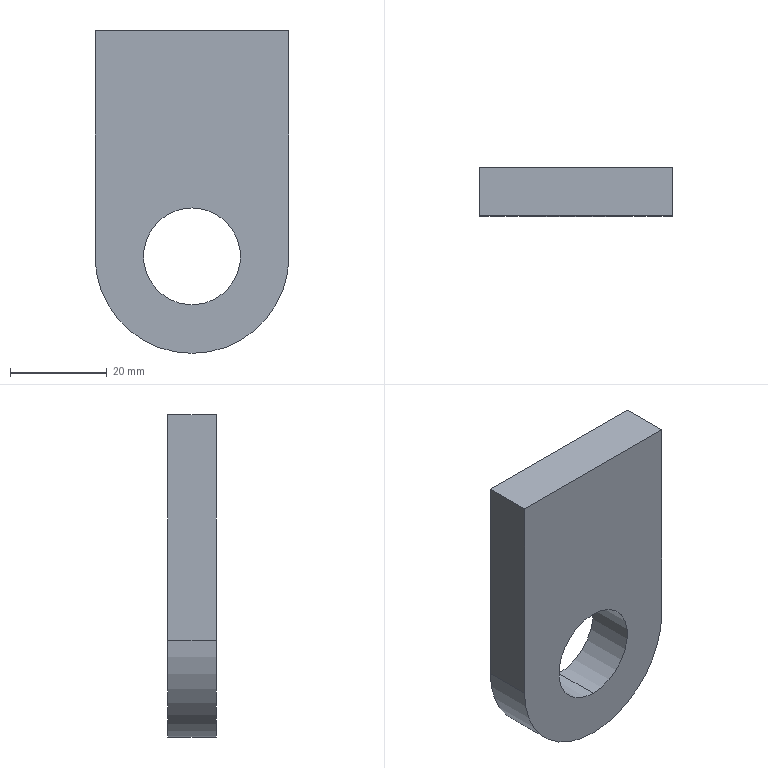Part | SolidWorks | features Extrusion 1 | 1 solid | 9 faces | box 40 x 10 x 66.57 mm | volume 21770 mm3 | plane 5 | cylinder 4 | commonest cylinder face diameters 20 x2 40 x2
STEP:
#1=CARTESIAN_POINT('',(0.,5.,-33.285));
#2=VERTEX_POINT('',#1);
#3=CARTESIAN_POINT('',(0.,5.,-13.285));
#4=VERTEX_POINT('',#3);
#5=CARTESIAN_POINT('',(0.,5.,-23.285));
#6=DIRECTION('',(0.,1.,0.));
#7=DIRECTION('',(0.,0.,1.));
#8=AXIS2_PLACEMENT_3D('',#5,#6,#7);
#9=CIRCLE('',#8,10.);
#10=EDGE_CURVE('',#2,#4,#9,.T.);
#11=ORIENTED_EDGE('',*,*,#10,.T.);
#12=CARTESIAN_POINT('',(0.,-5.,-13.285));
#13=VERTEX_POINT('',#12);
#14=CARTESIAN_POINT('',(0.,5.,-13.285));
#15=DIRECTION('',(0.,-1.,0.));
#16=VECTOR('',#15,1000.);
#17=LINE('',#14,#16);
#18=EDGE_CURVE('',#4,#13,#17,.T.);
#19=ORIENTED_EDGE('',*,*,#18,.T.);
#20=CARTESIAN_POINT('',(0.,-5.,-33.285));
#21=VERTEX_POINT('',#20);
#22=CARTESIAN_POINT('',(0.,-5.,-23.285));
#23=DIRECTION('',(0.,1.,0.));
#24=DIRECTION('',(0.,0.,1.));
#25=AXIS2_PLACEMENT_3D('',#22,#23,#24);
#26=CIRCLE('',#25,10.);
#27=EDGE_CURVE('',#21,#13,#26,.T.);
#28=ORIENTED_EDGE('',*,*,#27,.F.);
#29=CARTESIAN_POINT('',(0.,5.,-33.285));
#30=DIRECTION('',(0.,-1.,0.));
#31=VECTOR('',#30,1000.);
#32=LINE('',#29,#31);
#33=EDGE_CURVE('',#2,#21,#32,.T.);
#34=ORIENTED_EDGE('',*,*,#33,.F.);
#35=EDGE_LOOP('',(#11,#19,#28,#34));
#36=FACE_OUTER_BOUND('',#35,.T.);
#37=CARTESIAN_POINT('',(0.,5.,-23.285));
#38=DIRECTION('',(0.,-1.,0.));
#39=DIRECTION('',(0.,0.,-1.));
#40=AXIS2_PLACEMENT_3D('',#37,#38,#39);
#41=CYLINDRICAL_SURFACE('',#40,10.);
#42=ADVANCED_FACE('',(#36),#41,.F.);
#43=CARTESIAN_POINT('',(0.,5.,-43.285));
#44=VERTEX_POINT('',#43);
#45=CARTESIAN_POINT('',(-20.,5.,-23.285));
#46=VERTEX_POINT('',#45);
#47=CARTESIAN_POINT('',(0.,5.,-23.285));
#48=DIRECTION('',(0.,1.,0.));
#49=DIRECTION('',(0.,0.,1.));
#50=AXIS2_PLACEMENT_3D('',#47,#48,#49);
#51=CIRCLE('',#50,20.);
#52=EDGE_CURVE('',#44,#46,#51,.T.);
#53=ORIENTED_EDGE('',*,*,#52,.F.);
#54=CARTESIAN_POINT('',(0.,-5.,-43.285));
#55=VERTEX_POINT('',#54);
#56=CARTESIAN_POINT('',(0.,5.,-43.285));
#57=DIRECTION('',(0.,-1.,0.));
#58=VECTOR('',#57,1000.);
#59=LINE('',#56,#58);
#60=EDGE_CURVE('',#44,#55,#59,.T.);
#61=ORIENTED_EDGE('',*,*,#60,.T.);
#62=CARTESIAN_POINT('',(-20.,-5.,-23.285));
#63=VERTEX_POINT('',#62);
#64=CARTESIAN_POINT('',(0.,-5.,-23.285));
#65=DIRECTION('',(0.,1.,0.));
#66=DIRECTION('',(0.,0.,1.));
#67=AXIS2_PLACEMENT_3D('',#64,#65,#66);
#68=CIRCLE('',#67,20.);
#69=EDGE_CURVE('',#55,#63,#68,.T.);
#70=ORIENTED_EDGE('',*,*,#69,.T.);
#71=CARTESIAN_POINT('',(-20.,5.,-23.285));
#72=DIRECTION('',(0.,-1.,0.));
#73=VECTOR('',#72,1000.);
#74=LINE('',#71,#73);
#75=EDGE_CURVE('',#46,#63,#74,.T.);
#76=ORIENTED_EDGE('',*,*,#75,.F.);
#77=EDGE_LOOP('',(#53,#61,#70,#76));
#78=FACE_OUTER_BOUND('',#77,.T.);
#79=CARTESIAN_POINT('',(0.,5.,-23.285));
#80=DIRECTION('',(0.,-1.,0.));
#81=DIRECTION('',(0.,0.,-1.));
#82=AXIS2_PLACEMENT_3D('',#79,#80,#81);
#83=CYLINDRICAL_SURFACE('',#82,20.);
#84=ADVANCED_FACE('',(#78),#83,.T.);
#85=CARTESIAN_POINT('',(20.,5.,-23.285));
#86=VERTEX_POINT('',#85);
#87=CARTESIAN_POINT('',(0.,5.,-23.285));
#88=DIRECTION('',(0.,1.,0.));
#89=DIRECTION('',(0.,0.,1.));
#90=AXIS2_PLACEMENT_3D('',#87,#88,#89);
#91=CIRCLE('',#90,20.);
#92=EDGE_CURVE('',#86,#44,#91,.T.);
#93=ORIENTED_EDGE('',*,*,#92,.T.);
#94=ORIENTED_EDGE('',*,*,#52,.T.);
#95=CARTESIAN_POINT('',(-20.,5.,23.285));
#96=VERTEX_POINT('',#95);
#97=CARTESIAN_POINT('',(-20.,5.,23.285));
#98=DIRECTION('',(0.,0.,1.));
#99=VECTOR('',#98,1000.);
#100=LINE('',#97,#99);
#101=EDGE_CURVE('',#46,#96,#100,.T.);
#102=ORIENTED_EDGE('',*,*,#101,.T.);
#103=CARTESIAN_POINT('',(20.,5.,23.285));
#104=VERTEX_POINT('',#103);
#105=CARTESIAN_POINT('',(-20.,5.,23.285));
#106=DIRECTION('',(1.,0.,0.));
#107=VECTOR('',#106,1000.);
#108=LINE('',#105,#107);
#109=EDGE_CURVE('',#96,#104,#108,.T.);
#110=ORIENTED_EDGE('',*,*,#109,.T.);
#111=CARTESIAN_POINT('',(20.,5.,23.285));
#112=DIRECTION('',(0.,0.,-1.));
#113=VECTOR('',#112,1000.);
#114=LINE('',#111,#113);
#115=EDGE_CURVE('',#104,#86,#114,.T.);
#116=ORIENTED_EDGE('',*,*,#115,.T.);
#117=EDGE_LOOP('',(#93,#94,#102,#110,#116));
#118=FACE_OUTER_BOUND('',#117,.T.);
#119=ORIENTED_EDGE('',*,*,#10,.F.);
#120=CARTESIAN_POINT('',(0.,5.,-23.285));
#121=DIRECTION('',(0.,1.,0.));
#122=DIRECTION('',(0.,0.,1.));
#123=AXIS2_PLACEMENT_3D('',#120,#121,#122);
#124=CIRCLE('',#123,10.);
#125=EDGE_CURVE('',#4,#2,#124,.T.);
#126=ORIENTED_EDGE('',*,*,#125,.F.);
#127=EDGE_LOOP('',(#119,#126));
#128=FACE_BOUND('',#127,.T.);
#129=CARTESIAN_POINT('',(0.,5.,-23.285));
#130=DIRECTION('',(0.,1.,0.));
#131=DIRECTION('',(0.,0.,1.));
#132=AXIS2_PLACEMENT_3D('',#129,#130,#131);
#133=PLANE('',#132);
#134=ADVANCED_FACE('',(#118,#128),#133,.T.);
#135=CARTESIAN_POINT('',(20.,-5.,-23.285));
#136=VERTEX_POINT('',#135);
#137=CARTESIAN_POINT('',(0.,-5.,-23.285));
#138=DIRECTION('',(0.,1.,0.));
#139=DIRECTION('',(0.,0.,1.));
#140=AXIS2_PLACEMENT_3D('',#137,#138,#139);
#141=CIRCLE('',#140,20.);
#142=EDGE_CURVE('',#136,#55,#141,.T.);
#143=ORIENTED_EDGE('',*,*,#142,.F.);
#144=CARTESIAN_POINT('',(20.,-5.,23.285));
#145=VERTEX_POINT('',#144);
#146=CARTESIAN_POINT('',(20.,-5.,23.285));
#147=DIRECTION('',(0.,0.,-1.));
#148=VECTOR('',#147,1000.);
#149=LINE('',#146,#148);
#150=EDGE_CURVE('',#145,#136,#149,.T.);
#151=ORIENTED_EDGE('',*,*,#150,.F.);
#152=CARTESIAN_POINT('',(-20.,-5.,23.285));
#153=VERTEX_POINT('',#152);
#154=CARTESIAN_POINT('',(-20.,-5.,23.285));
#155=DIRECTION('',(1.,0.,0.));
#156=VECTOR('',#155,1000.);
#157=LINE('',#154,#156);
#158=EDGE_CURVE('',#153,#145,#157,.T.);
#159=ORIENTED_EDGE('',*,*,#158,.F.);
#160=CARTESIAN_POINT('',(-20.,-5.,23.285));
#161=DIRECTION('',(0.,0.,1.));
#162=VECTOR('',#161,1000.);
#163=LINE('',#160,#162);
#164=EDGE_CURVE('',#63,#153,#163,.T.);
#165=ORIENTED_EDGE('',*,*,#164,.F.);
#166=ORIENTED_EDGE('',*,*,#69,.F.);
#167=EDGE_LOOP('',(#143,#151,#159,#165,#166));
#168=FACE_OUTER_BOUND('',#167,.T.);
#169=ORIENTED_EDGE('',*,*,#27,.T.);
#170=CARTESIAN_POINT('',(0.,-5.,-23.285));
#171=DIRECTION('',(0.,1.,0.));
#172=DIRECTION('',(0.,0.,1.));
#173=AXIS2_PLACEMENT_3D('',#170,#171,#172);
#174=CIRCLE('',#173,10.);
#175=EDGE_CURVE('',#13,#21,#174,.T.);
#176=ORIENTED_EDGE('',*,*,#175,.T.);
#177=EDGE_LOOP('',(#169,#176));
#178=FACE_BOUND('',#177,.T.);
#179=CARTESIAN_POINT('',(0.,-5.,-23.285));
#180=DIRECTION('',(0.,1.,0.));
#181=DIRECTION('',(0.,0.,1.));
#182=AXIS2_PLACEMENT_3D('',#179,#180,#181);
#183=PLANE('',#182);
#184=ADVANCED_FACE('',(#168,#178),#183,.F.);
#185=ORIENTED_EDGE('',*,*,#60,.F.);
#186=ORIENTED_EDGE('',*,*,#92,.F.);
#187=CARTESIAN_POINT('',(20.,5.,-23.285));
#188=DIRECTION('',(0.,-1.,0.));
#189=VECTOR('',#188,1000.);
#190=LINE('',#187,#189);
#191=EDGE_CURVE('',#86,#136,#190,.T.);
#192=ORIENTED_EDGE('',*,*,#191,.T.);
#193=ORIENTED_EDGE('',*,*,#142,.T.);
#194=EDGE_LOOP('',(#185,#186,#192,#193));
#195=FACE_OUTER_BOUND('',#194,.T.);
#196=CARTESIAN_POINT('',(0.,5.,-23.285));
#197=DIRECTION('',(0.,-1.,0.));
#198=DIRECTION('',(0.,0.,-1.));
#199=AXIS2_PLACEMENT_3D('',#196,#197,#198);
#200=CYLINDRICAL_SURFACE('',#199,20.);
#201=ADVANCED_FACE('',(#195),#200,.T.);
#202=ORIENTED_EDGE('',*,*,#164,.T.);
#203=CARTESIAN_POINT('',(-20.,5.,23.285));
#204=DIRECTION('',(0.,-1.,0.));
#205=VECTOR('',#204,1000.);
#206=LINE('',#203,#205);
#207=EDGE_CURVE('',#96,#153,#206,.T.);
#208=ORIENTED_EDGE('',*,*,#207,.F.);
#209=ORIENTED_EDGE('',*,*,#101,.F.);
#210=ORIENTED_EDGE('',*,*,#75,.T.);
#211=EDGE_LOOP('',(#202,#208,#209,#210));
#212=FACE_OUTER_BOUND('',#211,.T.);
#213=CARTESIAN_POINT('',(-20.,5.,23.285));
#214=DIRECTION('',(1.,0.,0.));
#215=DIRECTION('',(0.,0.,-1.));
#216=AXIS2_PLACEMENT_3D('',#213,#214,#215);
#217=PLANE('',#216);
#218=ADVANCED_FACE('',(#212),#217,.F.);
#219=ORIENTED_EDGE('',*,*,#158,.T.);
#220=CARTESIAN_POINT('',(20.,5.,23.285));
#221=DIRECTION('',(0.,-1.,0.));
#222=VECTOR('',#221,1000.);
#223=LINE('',#220,#222);
#224=EDGE_CURVE('',#104,#145,#223,.T.);
#225=ORIENTED_EDGE('',*,*,#224,.F.);
#226=ORIENTED_EDGE('',*,*,#109,.F.);
#227=ORIENTED_EDGE('',*,*,#207,.T.);
#228=EDGE_LOOP('',(#219,#225,#226,#227));
#229=FACE_OUTER_BOUND('',#228,.T.);
#230=CARTESIAN_POINT('',(-20.,5.,23.285));
#231=DIRECTION('',(0.,0.,-1.));
#232=DIRECTION('',(-1.,0.,0.));
#233=AXIS2_PLACEMENT_3D('',#230,#231,#232);
#234=PLANE('',#233);
#235=ADVANCED_FACE('',(#229),#234,.F.);
#236=ORIENTED_EDGE('',*,*,#150,.T.);
#237=ORIENTED_EDGE('',*,*,#191,.F.);
#238=ORIENTED_EDGE('',*,*,#115,.F.);
#239=ORIENTED_EDGE('',*,*,#224,.T.);
#240=EDGE_LOOP('',(#236,#237,#238,#239));
#241=FACE_OUTER_BOUND('',#240,.T.);
#242=CARTESIAN_POINT('',(20.,5.,23.285));
#243=DIRECTION('',(-1.,0.,0.));
#244=DIRECTION('',(0.,0.,1.));
#245=AXIS2_PLACEMENT_3D('',#242,#243,#244);
#246=PLANE('',#245);
#247=ADVANCED_FACE('',(#241),#246,.F.);
#248=ORIENTED_EDGE('',*,*,#18,.F.);
#249=ORIENTED_EDGE('',*,*,#125,.T.);
#250=ORIENTED_EDGE('',*,*,#33,.T.);
#251=ORIENTED_EDGE('',*,*,#175,.F.);
#252=EDGE_LOOP('',(#248,#249,#250,#251));
#253=FACE_OUTER_BOUND('',#252,.T.);
#254=CARTESIAN_POINT('',(0.,5.,-23.285));
#255=DIRECTION('',(0.,-1.,0.));
#256=DIRECTION('',(0.,0.,-1.));
#257=AXIS2_PLACEMENT_3D('',#254,#255,#256);
#258=CYLINDRICAL_SURFACE('',#257,10.);
#259=ADVANCED_FACE('',(#253),#258,.F.);
#260=CLOSED_SHELL('',(#42,#84,#134,#184,#201,#218,#235,#247,#259));
#261=MANIFOLD_SOLID_BREP('',#260);
#262=CARTESIAN_POINT('',(0.,0.,0.));
#263=DIRECTION('',(0.,0.,1.));
#264=DIRECTION('',(1.,0.,0.));
#265=AXIS2_PLACEMENT_3D('',#262,#263,#264);
#266=(LENGTH_UNIT()NAMED_UNIT(*)SI_UNIT(.MILLI.,.METRE.));
#267=UNCERTAINTY_MEASURE_WITH_UNIT(LENGTH_MEASURE(0.00001),#266,'','');
#268=(NAMED_UNIT(*)PLANE_ANGLE_UNIT()SI_UNIT($,.RADIAN.));
#269=(NAMED_UNIT(*)SI_UNIT($,.STERADIAN.)SOLID_ANGLE_UNIT());
#270=(GEOMETRIC_REPRESENTATION_CONTEXT(3)GLOBAL_UNCERTAINTY_ASSIGNED_CONTEXT((#267))GLOBAL_UNIT_ASSIGNED_CONTEXT((#266,#268,#269))REPRESENTATION_CONTEXT('',''));
#271=ADVANCED_BREP_SHAPE_REPRESENTATION('',(#261,#265),#270);